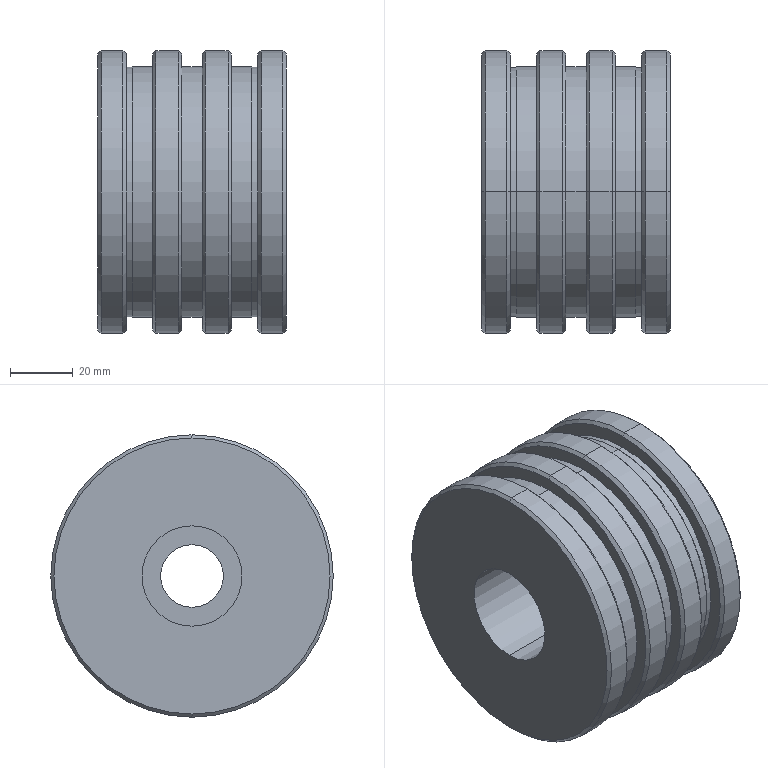Part | SolidWorks | features Chamfer 1, Revolution 1 | 1 solid | 52 faces | box 60 x 90 x 90 mm | volume 271909 mm3 | cylinder 24 | cone 16 | plane 12 | commonest cylinder face diameters 90 x8 80 x6 79.6 x4 20 x2 32 x2 64 x2
STEP:
#1=CARTESIAN_POINT('',(0.,0.,44.));
#2=VERTEX_POINT('',#1);
#3=CARTESIAN_POINT('',(0.,0.,-44.));
#4=VERTEX_POINT('',#3);
#5=CARTESIAN_POINT('',(0.,0.,0.));
#6=DIRECTION('',(-1.,0.,0.));
#7=DIRECTION('',(0.,0.,-1.));
#8=AXIS2_PLACEMENT_3D('',#5,#6,#7);
#9=CIRCLE('',#8,44.);
#10=EDGE_CURVE('',#2,#4,#9,.T.);
#11=ORIENTED_EDGE('',*,*,#10,.F.);
#12=CARTESIAN_POINT('',(1.,0.,45.));
#13=VERTEX_POINT('',#12);
#14=CARTESIAN_POINT('',(0.,0.,44.));
#15=DIRECTION('',(0.7071,0.,0.7071));
#16=VECTOR('',#15,1000.);
#17=LINE('',#14,#16);
#18=EDGE_CURVE('',#2,#13,#17,.T.);
#19=ORIENTED_EDGE('',*,*,#18,.T.);
#20=CARTESIAN_POINT('',(1.,0.,-45.));
#21=VERTEX_POINT('',#20);
#22=CARTESIAN_POINT('',(1.,0.,0.));
#23=DIRECTION('',(1.,0.,0.));
#24=DIRECTION('',(0.,0.,-1.));
#25=AXIS2_PLACEMENT_3D('',#22,#23,#24);
#26=CIRCLE('',#25,45.);
#27=EDGE_CURVE('',#21,#13,#26,.T.);
#28=ORIENTED_EDGE('',*,*,#27,.F.);
#29=CARTESIAN_POINT('',(0.,0.,-44.));
#30=DIRECTION('',(0.7071,0.,-0.7071));
#31=VECTOR('',#30,1000.);
#32=LINE('',#29,#31);
#33=EDGE_CURVE('',#4,#21,#32,.T.);
#34=ORIENTED_EDGE('',*,*,#33,.F.);
#35=EDGE_LOOP('',(#11,#19,#28,#34));
#36=FACE_OUTER_BOUND('',#35,.T.);
#37=CARTESIAN_POINT('',(0.,0.,0.));
#38=DIRECTION('',(1.,0.,0.));
#39=DIRECTION('',(0.,0.,-1.));
#40=AXIS2_PLACEMENT_3D('',#37,#38,#39);
#41=CONICAL_SURFACE('',#40,44.,0.7854);
#42=ADVANCED_FACE('',(#36),#41,.T.);
#43=CARTESIAN_POINT('',(9.,0.,-44.));
#44=VERTEX_POINT('',#43);
#45=CARTESIAN_POINT('',(9.,0.,44.));
#46=VERTEX_POINT('',#45);
#47=CARTESIAN_POINT('',(9.,0.,0.));
#48=DIRECTION('',(1.,0.,0.));
#49=DIRECTION('',(0.,0.,1.));
#50=AXIS2_PLACEMENT_3D('',#47,#48,#49);
#51=CIRCLE('',#50,44.);
#52=EDGE_CURVE('',#44,#46,#51,.T.);
#53=ORIENTED_EDGE('',*,*,#52,.F.);
#54=CARTESIAN_POINT('',(8.,0.,-45.));
#55=VERTEX_POINT('',#54);
#56=CARTESIAN_POINT('',(8.,0.,-45.));
#57=DIRECTION('',(-0.7071,0.,-0.7071));
#58=VECTOR('',#57,1000.);
#59=LINE('',#56,#58);
#60=EDGE_CURVE('',#44,#55,#59,.T.);
#61=ORIENTED_EDGE('',*,*,#60,.T.);
#62=CARTESIAN_POINT('',(8.,0.,45.));
#63=VERTEX_POINT('',#62);
#64=CARTESIAN_POINT('',(8.,0.,0.));
#65=DIRECTION('',(-1.,0.,0.));
#66=DIRECTION('',(0.,0.,1.));
#67=AXIS2_PLACEMENT_3D('',#64,#65,#66);
#68=CIRCLE('',#67,45.);
#69=EDGE_CURVE('',#63,#55,#68,.T.);
#70=ORIENTED_EDGE('',*,*,#69,.F.);
#71=CARTESIAN_POINT('',(8.,0.,45.));
#72=DIRECTION('',(-0.7071,0.,0.7071));
#73=VECTOR('',#72,1000.);
#74=LINE('',#71,#73);
#75=EDGE_CURVE('',#46,#63,#74,.T.);
#76=ORIENTED_EDGE('',*,*,#75,.F.);
#77=EDGE_LOOP('',(#53,#61,#70,#76));
#78=FACE_OUTER_BOUND('',#77,.T.);
#79=CARTESIAN_POINT('',(8.,0.,0.));
#80=DIRECTION('',(-1.,0.,0.));
#81=DIRECTION('',(0.,0.,1.));
#82=AXIS2_PLACEMENT_3D('',#79,#80,#81);
#83=CONICAL_SURFACE('',#82,45.,0.7854);
#84=ADVANCED_FACE('',(#78),#83,.T.);
#85=CARTESIAN_POINT('',(17.5,0.,44.));
#86=VERTEX_POINT('',#85);
#87=CARTESIAN_POINT('',(17.5,0.,-44.));
#88=VERTEX_POINT('',#87);
#89=CARTESIAN_POINT('',(17.5,0.,0.));
#90=DIRECTION('',(-1.,0.,0.));
#91=DIRECTION('',(0.,0.,-1.));
#92=AXIS2_PLACEMENT_3D('',#89,#90,#91);
#93=CIRCLE('',#92,44.);
#94=EDGE_CURVE('',#86,#88,#93,.T.);
#95=ORIENTED_EDGE('',*,*,#94,.F.);
#96=CARTESIAN_POINT('',(18.5,0.,45.));
#97=VERTEX_POINT('',#96);
#98=CARTESIAN_POINT('',(17.5,0.,44.));
#99=DIRECTION('',(0.7071,0.,0.7071));
#100=VECTOR('',#99,1000.);
#101=LINE('',#98,#100);
#102=EDGE_CURVE('',#86,#97,#101,.T.);
#103=ORIENTED_EDGE('',*,*,#102,.T.);
#104=CARTESIAN_POINT('',(18.5,0.,-45.));
#105=VERTEX_POINT('',#104);
#106=CARTESIAN_POINT('',(18.5,0.,0.));
#107=DIRECTION('',(1.,0.,0.));
#108=DIRECTION('',(0.,0.,-1.));
#109=AXIS2_PLACEMENT_3D('',#106,#107,#108);
#110=CIRCLE('',#109,45.);
#111=EDGE_CURVE('',#105,#97,#110,.T.);
#112=ORIENTED_EDGE('',*,*,#111,.F.);
#113=CARTESIAN_POINT('',(17.5,0.,-44.));
#114=DIRECTION('',(0.7071,0.,-0.7071));
#115=VECTOR('',#114,1000.);
#116=LINE('',#113,#115);
#117=EDGE_CURVE('',#88,#105,#116,.T.);
#118=ORIENTED_EDGE('',*,*,#117,.F.);
#119=EDGE_LOOP('',(#95,#103,#112,#118));
#120=FACE_OUTER_BOUND('',#119,.T.);
#121=CARTESIAN_POINT('',(17.5,0.,0.));
#122=DIRECTION('',(1.,0.,0.));
#123=DIRECTION('',(0.,0.,-1.));
#124=AXIS2_PLACEMENT_3D('',#121,#122,#123);
#125=CONICAL_SURFACE('',#124,44.,0.7854);
#126=ADVANCED_FACE('',(#120),#125,.T.);
#127=CARTESIAN_POINT('',(26.75,0.,-44.));
#128=VERTEX_POINT('',#127);
#129=CARTESIAN_POINT('',(26.75,0.,44.));
#130=VERTEX_POINT('',#129);
#131=CARTESIAN_POINT('',(26.75,0.,0.));
#132=DIRECTION('',(1.,0.,0.));
#133=DIRECTION('',(0.,0.,1.));
#134=AXIS2_PLACEMENT_3D('',#131,#132,#133);
#135=CIRCLE('',#134,44.);
#136=EDGE_CURVE('',#128,#130,#135,.T.);
#137=ORIENTED_EDGE('',*,*,#136,.F.);
#138=CARTESIAN_POINT('',(25.75,0.,-45.));
#139=VERTEX_POINT('',#138);
#140=CARTESIAN_POINT('',(25.75,0.,-45.));
#141=DIRECTION('',(-0.7071,0.,-0.7071));
#142=VECTOR('',#141,1000.);
#143=LINE('',#140,#142);
#144=EDGE_CURVE('',#128,#139,#143,.T.);
#145=ORIENTED_EDGE('',*,*,#144,.T.);
#146=CARTESIAN_POINT('',(25.75,0.,45.));
#147=VERTEX_POINT('',#146);
#148=CARTESIAN_POINT('',(25.75,0.,0.));
#149=DIRECTION('',(-1.,0.,0.));
#150=DIRECTION('',(0.,0.,1.));
#151=AXIS2_PLACEMENT_3D('',#148,#149,#150);
#152=CIRCLE('',#151,45.);
#153=EDGE_CURVE('',#147,#139,#152,.T.);
#154=ORIENTED_EDGE('',*,*,#153,.F.);
#155=CARTESIAN_POINT('',(25.75,0.,45.));
#156=DIRECTION('',(-0.7071,0.,0.7071));
#157=VECTOR('',#156,1000.);
#158=LINE('',#155,#157);
#159=EDGE_CURVE('',#130,#147,#158,.T.);
#160=ORIENTED_EDGE('',*,*,#159,.F.);
#161=EDGE_LOOP('',(#137,#145,#154,#160));
#162=FACE_OUTER_BOUND('',#161,.T.);
#163=CARTESIAN_POINT('',(25.75,0.,0.));
#164=DIRECTION('',(-1.,0.,0.));
#165=DIRECTION('',(0.,0.,1.));
#166=AXIS2_PLACEMENT_3D('',#163,#164,#165);
#167=CONICAL_SURFACE('',#166,45.,0.7854);
#168=ADVANCED_FACE('',(#162),#167,.T.);
#169=CARTESIAN_POINT('',(33.25,0.,44.));
#170=VERTEX_POINT('',#169);
#171=CARTESIAN_POINT('',(33.25,0.,-44.));
#172=VERTEX_POINT('',#171);
#173=CARTESIAN_POINT('',(33.25,0.,0.));
#174=DIRECTION('',(-1.,0.,0.));
#175=DIRECTION('',(0.,0.,-1.));
#176=AXIS2_PLACEMENT_3D('',#173,#174,#175);
#177=CIRCLE('',#176,44.);
#178=EDGE_CURVE('',#170,#172,#177,.T.);
#179=ORIENTED_EDGE('',*,*,#178,.F.);
#180=CARTESIAN_POINT('',(34.25,0.,45.));
#181=VERTEX_POINT('',#180);
#182=CARTESIAN_POINT('',(33.25,0.,44.));
#183=DIRECTION('',(0.7071,0.,0.7071));
#184=VECTOR('',#183,1000.);
#185=LINE('',#182,#184);
#186=EDGE_CURVE('',#170,#181,#185,.T.);
#187=ORIENTED_EDGE('',*,*,#186,.T.);
#188=CARTESIAN_POINT('',(34.25,0.,-45.));
#189=VERTEX_POINT('',#188);
#190=CARTESIAN_POINT('',(34.25,0.,0.));
#191=DIRECTION('',(1.,0.,0.));
#192=DIRECTION('',(0.,0.,-1.));
#193=AXIS2_PLACEMENT_3D('',#190,#191,#192);
#194=CIRCLE('',#193,45.);
#195=EDGE_CURVE('',#189,#181,#194,.T.);
#196=ORIENTED_EDGE('',*,*,#195,.F.);
#197=CARTESIAN_POINT('',(33.25,0.,-44.));
#198=DIRECTION('',(0.7071,0.,-0.7071));
#199=VECTOR('',#198,1000.);
#200=LINE('',#197,#199);
#201=EDGE_CURVE('',#172,#189,#200,.T.);
#202=ORIENTED_EDGE('',*,*,#201,.F.);
#203=EDGE_LOOP('',(#179,#187,#196,#202));
#204=FACE_OUTER_BOUND('',#203,.T.);
#205=CARTESIAN_POINT('',(33.25,0.,0.));
#206=DIRECTION('',(1.,0.,0.));
#207=DIRECTION('',(0.,0.,-1.));
#208=AXIS2_PLACEMENT_3D('',#205,#206,#207);
#209=CONICAL_SURFACE('',#208,44.,0.7854);
#210=ADVANCED_FACE('',(#204),#209,.T.);
#211=CARTESIAN_POINT('',(42.5,0.,-44.));
#212=VERTEX_POINT('',#211);
#213=CARTESIAN_POINT('',(42.5,0.,44.));
#214=VERTEX_POINT('',#213);
#215=CARTESIAN_POINT('',(42.5,0.,0.));
#216=DIRECTION('',(1.,0.,0.));
#217=DIRECTION('',(0.,0.,1.));
#218=AXIS2_PLACEMENT_3D('',#215,#216,#217);
#219=CIRCLE('',#218,44.);
#220=EDGE_CURVE('',#212,#214,#219,.T.);
#221=ORIENTED_EDGE('',*,*,#220,.F.);
#222=CARTESIAN_POINT('',(41.5,0.,-45.));
#223=VERTEX_POINT('',#222);
#224=CARTESIAN_POINT('',(41.5,0.,-45.));
#225=DIRECTION('',(-0.7071,0.,-0.7071));
#226=VECTOR('',#225,1000.);
#227=LINE('',#224,#226);
#228=EDGE_CURVE('',#212,#223,#227,.T.);
#229=ORIENTED_EDGE('',*,*,#228,.T.);
#230=CARTESIAN_POINT('',(41.5,0.,45.));
#231=VERTEX_POINT('',#230);
#232=CARTESIAN_POINT('',(41.5,0.,0.));
#233=DIRECTION('',(-1.,0.,0.));
#234=DIRECTION('',(0.,0.,1.));
#235=AXIS2_PLACEMENT_3D('',#232,#233,#234);
#236=CIRCLE('',#235,45.);
#237=EDGE_CURVE('',#231,#223,#236,.T.);
#238=ORIENTED_EDGE('',*,*,#237,.F.);
#239=CARTESIAN_POINT('',(41.5,0.,45.));
#240=DIRECTION('',(-0.7071,0.,0.7071));
#241=VECTOR('',#240,1000.);
#242=LINE('',#239,#241);
#243=EDGE_CURVE('',#214,#231,#242,.T.);
#244=ORIENTED_EDGE('',*,*,#243,.F.);
#245=EDGE_LOOP('',(#221,#229,#238,#244));
#246=FACE_OUTER_BOUND('',#245,.T.);
#247=CARTESIAN_POINT('',(41.5,0.,0.));
#248=DIRECTION('',(-1.,0.,0.));
#249=DIRECTION('',(0.,0.,1.));
#250=AXIS2_PLACEMENT_3D('',#247,#248,#249);
#251=CONICAL_SURFACE('',#250,45.,0.7854);
#252=ADVANCED_FACE('',(#246),#251,.T.);
#253=CARTESIAN_POINT('',(51.,0.,44.));
#254=VERTEX_POINT('',#253);
#255=CARTESIAN_POINT('',(51.,0.,-44.));
#256=VERTEX_POINT('',#255);
#257=CARTESIAN_POINT('',(51.,0.,0.));
#258=DIRECTION('',(-1.,0.,0.));
#259=DIRECTION('',(0.,0.,-1.));
#260=AXIS2_PLACEMENT_3D('',#257,#258,#259);
#261=CIRCLE('',#260,44.);
#262=EDGE_CURVE('',#254,#256,#261,.T.);
#263=ORIENTED_EDGE('',*,*,#262,.F.);
#264=CARTESIAN_POINT('',(52.,0.,45.));
#265=VERTEX_POINT('',#264);
#266=CARTESIAN_POINT('',(51.,0.,44.));
#267=DIRECTION('',(0.7071,0.,0.7071));
#268=VECTOR('',#267,1000.);
#269=LINE('',#266,#268);
#270=EDGE_CURVE('',#254,#265,#269,.T.);
#271=ORIENTED_EDGE('',*,*,#270,.T.);
#272=CARTESIAN_POINT('',(52.,0.,-45.));
#273=VERTEX_POINT('',#272);
#274=CARTESIAN_POINT('',(52.,0.,0.));
#275=DIRECTION('',(1.,0.,0.));
#276=DIRECTION('',(0.,0.,-1.));
#277=AXIS2_PLACEMENT_3D('',#274,#275,#276);
#278=CIRCLE('',#277,45.);
#279=EDGE_CURVE('',#273,#265,#278,.T.);
#280=ORIENTED_EDGE('',*,*,#279,.F.);
#281=CARTESIAN_POINT('',(51.,0.,-44.));
#282=DIRECTION('',(0.7071,0.,-0.7071));
#283=VECTOR('',#282,1000.);
#284=LINE('',#281,#283);
#285=EDGE_CURVE('',#256,#273,#284,.T.);
#286=ORIENTED_EDGE('',*,*,#285,.F.);
#287=EDGE_LOOP('',(#263,#271,#280,#286));
#288=FACE_OUTER_BOUND('',#287,.T.);
#289=CARTESIAN_POINT('',(51.,0.,0.));
#290=DIRECTION('',(1.,0.,0.));
#291=DIRECTION('',(0.,0.,-1.));
#292=AXIS2_PLACEMENT_3D('',#289,#290,#291);
#293=CONICAL_SURFACE('',#292,44.,0.7854);
#294=ADVANCED_FACE('',(#288),#293,.T.);
#295=CARTESIAN_POINT('',(60.,0.,-44.));
#296=VERTEX_POINT('',#295);
#297=CARTESIAN_POINT('',(60.,0.,44.));
#298=VERTEX_POINT('',#297);
#299=CARTESIAN_POINT('',(60.,0.,0.));
#300=DIRECTION('',(1.,0.,0.));
#301=DIRECTION('',(0.,0.,1.));
#302=AXIS2_PLACEMENT_3D('',#299,#300,#301);
#303=CIRCLE('',#302,44.);
#304=EDGE_CURVE('',#296,#298,#303,.T.);
#305=ORIENTED_EDGE('',*,*,#304,.F.);
#306=CARTESIAN_POINT('',(59.,0.,-45.));
#307=VERTEX_POINT('',#306);
#308=CARTESIAN_POINT('',(59.,0.,-45.));
#309=DIRECTION('',(-0.7071,0.,-0.7071));
#310=VECTOR('',#309,1000.);
#311=LINE('',#308,#310);
#312=EDGE_CURVE('',#296,#307,#311,.T.);
#313=ORIENTED_EDGE('',*,*,#312,.T.);
#314=CARTESIAN_POINT('',(59.,0.,45.));
#315=VERTEX_POINT('',#314);
#316=CARTESIAN_POINT('',(59.,0.,0.));
#317=DIRECTION('',(-1.,0.,0.));
#318=DIRECTION('',(0.,0.,1.));
#319=AXIS2_PLACEMENT_3D('',#316,#317,#318);
#320=CIRCLE('',#319,45.);
#321=EDGE_CURVE('',#315,#307,#320,.T.);
#322=ORIENTED_EDGE('',*,*,#321,.F.);
#323=CARTESIAN_POINT('',(59.,0.,45.));
#324=DIRECTION('',(-0.7071,0.,0.7071));
#325=VECTOR('',#324,1000.);
#326=LINE('',#323,#325);
#327=EDGE_CURVE('',#298,#315,#326,.T.);
#328=ORIENTED_EDGE('',*,*,#327,.F.);
#329=EDGE_LOOP('',(#305,#313,#322,#328));
#330=FACE_OUTER_BOUND('',#329,.T.);
#331=CARTESIAN_POINT('',(59.,0.,0.));
#332=DIRECTION('',(-1.,0.,0.));
#333=DIRECTION('',(0.,0.,1.));
#334=AXIS2_PLACEMENT_3D('',#331,#332,#333);
#335=CONICAL_SURFACE('',#334,45.,0.7854);
#336=ADVANCED_FACE('',(#330),#335,.T.);
#337=CARTESIAN_POINT('',(45.,0.,-10.));
#338=VERTEX_POINT('',#337);
#339=CARTESIAN_POINT('',(45.,0.,10.));
#340=VERTEX_POINT('',#339);
#341=CARTESIAN_POINT('',(45.,0.,0.));
#342=DIRECTION('',(-1.,0.,0.));
#343=DIRECTION('',(0.,0.,1.));
#344=AXIS2_PLACEMENT_3D('',#341,#342,#343);
#345=CIRCLE('',#344,10.);
#346=EDGE_CURVE('',#338,#340,#345,.T.);
#347=ORIENTED_EDGE('',*,*,#346,.F.);
#348=CARTESIAN_POINT('',(30.,0.,-10.));
#349=VERTEX_POINT('',#348);
#350=CARTESIAN_POINT('',(0.,0.,-10.));
#351=DIRECTION('',(-1.,0.,0.));
#352=VECTOR('',#351,1000.);
#353=LINE('',#350,#352);
#354=EDGE_CURVE('',#338,#349,#353,.T.);
#355=ORIENTED_EDGE('',*,*,#354,.T.);
#356=CARTESIAN_POINT('',(30.,0.,10.));
#357=VERTEX_POINT('',#356);
#358=CARTESIAN_POINT('',(30.,0.,0.));
#359=DIRECTION('',(-1.,0.,0.));
#360=DIRECTION('',(0.,0.,1.));
#361=AXIS2_PLACEMENT_3D('',#358,#359,#360);
#362=CIRCLE('',#361,10.);
#363=EDGE_CURVE('',#349,#357,#362,.T.);
#364=ORIENTED_EDGE('',*,*,#363,.T.);
#365=CARTESIAN_POINT('',(0.,0.,10.));
#366=DIRECTION('',(-1.,0.,0.));
#367=VECTOR('',#366,1000.);
#368=LINE('',#365,#367);
#369=EDGE_CURVE('',#340,#357,#368,.T.);
#370=ORIENTED_EDGE('',*,*,#369,.F.);
#371=EDGE_LOOP('',(#347,#355,#364,#370));
#372=FACE_OUTER_BOUND('',#371,.T.);
#373=CARTESIAN_POINT('',(0.,0.,0.));
#374=DIRECTION('',(-1.,0.,0.));
#375=DIRECTION('',(0.,0.,1.));
#376=AXIS2_PLACEMENT_3D('',#373,#374,#375);
#377=CYLINDRICAL_SURFACE('',#376,10.);
#378=ADVANCED_FACE('',(#372),#377,.F.);
#379=CARTESIAN_POINT('',(60.,0.,-32.));
#380=VERTEX_POINT('',#379);
#381=CARTESIAN_POINT('',(60.,0.,32.));
#382=VERTEX_POINT('',#381);
#383=CARTESIAN_POINT('',(60.,0.,0.));
#384=DIRECTION('',(-1.,0.,0.));
#385=DIRECTION('',(0.,0.,1.));
#386=AXIS2_PLACEMENT_3D('',#383,#384,#385);
#387=CIRCLE('',#386,32.);
#388=EDGE_CURVE('',#380,#382,#387,.T.);
#389=ORIENTED_EDGE('',*,*,#388,.F.);
#390=CARTESIAN_POINT('',(45.,0.,-32.));
#391=VERTEX_POINT('',#390);
#392=CARTESIAN_POINT('',(0.,0.,-32.));
#393=DIRECTION('',(-1.,0.,0.));
#394=VECTOR('',#393,1000.);
#395=LINE('',#392,#394);
#396=EDGE_CURVE('',#380,#391,#395,.T.);
#397=ORIENTED_EDGE('',*,*,#396,.T.);
#398=CARTESIAN_POINT('',(45.,0.,32.));
#399=VERTEX_POINT('',#398);
#400=CARTESIAN_POINT('',(45.,0.,0.));
#401=DIRECTION('',(-1.,0.,0.));
#402=DIRECTION('',(0.,0.,1.));
#403=AXIS2_PLACEMENT_3D('',#400,#401,#402);
#404=CIRCLE('',#403,32.);
#405=EDGE_CURVE('',#391,#399,#404,.T.);
#406=ORIENTED_EDGE('',*,*,#405,.T.);
#407=CARTESIAN_POINT('',(0.,0.,32.));
#408=DIRECTION('',(-1.,0.,0.));
#409=VECTOR('',#408,1000.);
#410=LINE('',#407,#409);
#411=EDGE_CURVE('',#382,#399,#410,.T.);
#412=ORIENTED_EDGE('',*,*,#411,.F.);
#413=EDGE_LOOP('',(#389,#397,#406,#412));
#414=FACE_OUTER_BOUND('',#413,.T.);
#415=CARTESIAN_POINT('',(0.,0.,0.));
#416=DIRECTION('',(-1.,0.,0.));
#417=DIRECTION('',(0.,0.,1.));
#418=AXIS2_PLACEMENT_3D('',#415,#416,#417);
#419=CYLINDRICAL_SURFACE('',#418,32.);
#420=ADVANCED_FACE('',(#414),#419,.F.);
#421=ORIENTED_EDGE('',*,*,#321,.T.);
#422=CARTESIAN_POINT('',(0.,0.,-45.));
#423=DIRECTION('',(-1.,0.,0.));
#424=VECTOR('',#423,1000.);
#425=LINE('',#422,#424);
#426=EDGE_CURVE('',#307,#273,#425,.T.);
#427=ORIENTED_EDGE('',*,*,#426,.T.);
#428=ORIENTED_EDGE('',*,*,#279,.T.);
#429=CARTESIAN_POINT('',(0.,0.,45.));
#430=DIRECTION('',(-1.,0.,0.));
#431=VECTOR('',#430,1000.);
#432=LINE('',#429,#431);
#433=EDGE_CURVE('',#315,#265,#432,.T.);
#434=ORIENTED_EDGE('',*,*,#433,.F.);
#435=EDGE_LOOP('',(#421,#427,#428,#434));
#436=FACE_OUTER_BOUND('',#435,.T.);
#437=CARTESIAN_POINT('',(0.,0.,0.));
#438=DIRECTION('',(-1.,0.,0.));
#439=DIRECTION('',(0.,0.,1.));
#440=AXIS2_PLACEMENT_3D('',#437,#438,#439);
#441=CYLINDRICAL_SURFACE('',#440,45.);
#442=ADVANCED_FACE('',(#436),#441,.T.);
#443=CARTESIAN_POINT('',(51.,0.,39.8));
#444=VERTEX_POINT('',#443);
#445=CARTESIAN_POINT('',(51.,0.,-39.8));
#446=VERTEX_POINT('',#445);
#447=CARTESIAN_POINT('',(51.,0.,0.));
#448=DIRECTION('',(-1.,0.,0.));
#449=DIRECTION('',(0.,0.,1.));
#450=AXIS2_PLACEMENT_3D('',#447,#448,#449);
#451=CIRCLE('',#450,39.8);
#452=EDGE_CURVE('',#444,#446,#451,.T.);
#453=ORIENTED_EDGE('',*,*,#452,.T.);
#454=CARTESIAN_POINT('',(49.,0.,-39.8));
#455=VERTEX_POINT('',#454);
#456=CARTESIAN_POINT('',(0.,0.,-39.8));
#457=DIRECTION('',(-1.,0.,0.));
#458=VECTOR('',#457,1000.);
#459=LINE('',#456,#458);
#460=EDGE_CURVE('',#446,#455,#459,.T.);
#461=ORIENTED_EDGE('',*,*,#460,.T.);
#462=CARTESIAN_POINT('',(49.,0.,39.8));
#463=VERTEX_POINT('',#462);
#464=CARTESIAN_POINT('',(49.,0.,0.));
#465=DIRECTION('',(-1.,0.,0.));
#466=DIRECTION('',(0.,0.,1.));
#467=AXIS2_PLACEMENT_3D('',#464,#465,#466);
#468=CIRCLE('',#467,39.8);
#469=EDGE_CURVE('',#463,#455,#468,.T.);
#470=ORIENTED_EDGE('',*,*,#469,.F.);
#471=CARTESIAN_POINT('',(0.,0.,39.8));
#472=DIRECTION('',(-1.,0.,0.));
#473=VECTOR('',#472,1000.);
#474=LINE('',#471,#473);
#475=EDGE_CURVE('',#444,#463,#474,.T.);
#476=ORIENTED_EDGE('',*,*,#475,.F.);
#477=EDGE_LOOP('',(#453,#461,#470,#476));
#478=FACE_OUTER_BOUND('',#477,.T.);
#479=CARTESIAN_POINT('',(0.,0.,0.));
#480=DIRECTION('',(-1.,0.,0.));
#481=DIRECTION('',(0.,0.,1.));
#482=AXIS2_PLACEMENT_3D('',#479,#480,#481);
#483=CYLINDRICAL_SURFACE('',#482,39.8);
#484=ADVANCED_FACE('',(#478),#483,.T.);
#485=CARTESIAN_POINT('',(49.,0.,40.));
#486=VERTEX_POINT('',#485);
#487=CARTESIAN_POINT('',(49.,0.,-40.));
#488=VERTEX_POINT('',#487);
#489=CARTESIAN_POINT('',(49.,0.,0.));
#490=DIRECTION('',(-1.,0.,0.));
#491=DIRECTION('',(0.,0.,1.));
#492=AXIS2_PLACEMENT_3D('',#489,#490,#491);
#493=CIRCLE('',#492,40.);
#494=EDGE_CURVE('',#486,#488,#493,.T.);
#495=ORIENTED_EDGE('',*,*,#494,.T.);
#496=CARTESIAN_POINT('',(42.5,0.,-40.));
#497=VERTEX_POINT('',#496);
#498=CARTESIAN_POINT('',(0.,0.,-40.));
#499=DIRECTION('',(-1.,0.,0.));
#500=VECTOR('',#499,1000.);
#501=LINE('',#498,#500);
#502=EDGE_CURVE('',#488,#497,#501,.T.);
#503=ORIENTED_EDGE('',*,*,#502,.T.);
#504=CARTESIAN_POINT('',(42.5,0.,40.));
#505=VERTEX_POINT('',#504);
#506=CARTESIAN_POINT('',(42.5,0.,0.));
#507=DIRECTION('',(-1.,0.,0.));
#508=DIRECTION('',(0.,0.,1.));
#509=AXIS2_PLACEMENT_3D('',#506,#507,#508);
#510=CIRCLE('',#509,40.);
#511=EDGE_CURVE('',#505,#497,#510,.T.);
#512=ORIENTED_EDGE('',*,*,#511,.F.);
#513=CARTESIAN_POINT('',(0.,0.,40.));
#514=DIRECTION('',(-1.,0.,0.));
#515=VECTOR('',#514,1000.);
#516=LINE('',#513,#515);
#517=EDGE_CURVE('',#486,#505,#516,.T.);
#518=ORIENTED_EDGE('',*,*,#517,.F.);
#519=EDGE_LOOP('',(#495,#503,#512,#518));
#520=FACE_OUTER_BOUND('',#519,.T.);
#521=CARTESIAN_POINT('',(0.,0.,0.));
#522=DIRECTION('',(-1.,0.,0.));
#523=DIRECTION('',(0.,0.,1.));
#524=AXIS2_PLACEMENT_3D('',#521,#522,#523);
#525=CYLINDRICAL_SURFACE('',#524,40.);
#526=ADVANCED_FACE('',(#520),#525,.T.);
#527=ORIENTED_EDGE('',*,*,#237,.T.);
#528=CARTESIAN_POINT('',(0.,0.,-45.));
#529=DIRECTION('',(-1.,0.,0.));
#530=VECTOR('',#529,1000.);
#531=LINE('',#528,#530);
#532=EDGE_CURVE('',#223,#189,#531,.T.);
#533=ORIENTED_EDGE('',*,*,#532,.T.);
#534=ORIENTED_EDGE('',*,*,#195,.T.);
#535=CARTESIAN_POINT('',(0.,0.,45.));
#536=DIRECTION('',(-1.,0.,0.));
#537=VECTOR('',#536,1000.);
#538=LINE('',#535,#537);
#539=EDGE_CURVE('',#231,#181,#538,.T.);
#540=ORIENTED_EDGE('',*,*,#539,.F.);
#541=EDGE_LOOP('',(#527,#533,#534,#540));
#542=FACE_OUTER_BOUND('',#541,.T.);
#543=CARTESIAN_POINT('',(0.,0.,0.));
#544=DIRECTION('',(-1.,0.,0.));
#545=DIRECTION('',(0.,0.,1.));
#546=AXIS2_PLACEMENT_3D('',#543,#544,#545);
#547=CYLINDRICAL_SURFACE('',#546,45.);
#548=ADVANCED_FACE('',(#542),#547,.T.);
#549=CARTESIAN_POINT('',(33.25,0.,40.));
#550=VERTEX_POINT('',#549);
#551=CARTESIAN_POINT('',(33.25,0.,-40.));
#552=VERTEX_POINT('',#551);
#553=CARTESIAN_POINT('',(33.25,0.,0.));
#554=DIRECTION('',(-1.,0.,0.));
#555=DIRECTION('',(0.,0.,1.));
#556=AXIS2_PLACEMENT_3D('',#553,#554,#555);
#557=CIRCLE('',#556,40.);
#558=EDGE_CURVE('',#550,#552,#557,.T.);
#559=ORIENTED_EDGE('',*,*,#558,.T.);
#560=CARTESIAN_POINT('',(26.75,0.,-40.));
#561=VERTEX_POINT('',#560);
#562=CARTESIAN_POINT('',(0.,0.,-40.));
#563=DIRECTION('',(-1.,0.,0.));
#564=VECTOR('',#563,1000.);
#565=LINE('',#562,#564);
#566=EDGE_CURVE('',#552,#561,#565,.T.);
#567=ORIENTED_EDGE('',*,*,#566,.T.);
#568=CARTESIAN_POINT('',(26.75,0.,40.));
#569=VERTEX_POINT('',#568);
#570=CARTESIAN_POINT('',(26.75,0.,0.));
#571=DIRECTION('',(-1.,0.,0.));
#572=DIRECTION('',(0.,0.,1.));
#573=AXIS2_PLACEMENT_3D('',#570,#571,#572);
#574=CIRCLE('',#573,40.);
#575=EDGE_CURVE('',#569,#561,#574,.T.);
#576=ORIENTED_EDGE('',*,*,#575,.F.);
#577=CARTESIAN_POINT('',(0.,0.,40.));
#578=DIRECTION('',(-1.,0.,0.));
#579=VECTOR('',#578,1000.);
#580=LINE('',#577,#579);
#581=EDGE_CURVE('',#550,#569,#580,.T.);
#582=ORIENTED_EDGE('',*,*,#581,.F.);
#583=EDGE_LOOP('',(#559,#567,#576,#582));
#584=FACE_OUTER_BOUND('',#583,.T.);
#585=CARTESIAN_POINT('',(0.,0.,0.));
#586=DIRECTION('',(-1.,0.,0.));
#587=DIRECTION('',(0.,0.,1.));
#588=AXIS2_PLACEMENT_3D('',#585,#586,#587);
#589=CYLINDRICAL_SURFACE('',#588,40.);
#590=ADVANCED_FACE('',(#584),#589,.T.);
#591=ORIENTED_EDGE('',*,*,#153,.T.);
#592=CARTESIAN_POINT('',(0.,0.,-45.));
#593=DIRECTION('',(-1.,0.,0.));
#594=VECTOR('',#593,1000.);
#595=LINE('',#592,#594);
#596=EDGE_CURVE('',#139,#105,#595,.T.);
#597=ORIENTED_EDGE('',*,*,#596,.T.);
#598=ORIENTED_EDGE('',*,*,#111,.T.);
#599=CARTESIAN_POINT('',(0.,0.,45.));
#600=DIRECTION('',(-1.,0.,0.));
#601=VECTOR('',#600,1000.);
#602=LINE('',#599,#601);
#603=EDGE_CURVE('',#147,#97,#602,.T.);
#604=ORIENTED_EDGE('',*,*,#603,.F.);
#605=EDGE_LOOP('',(#591,#597,#598,#604));
#606=FACE_OUTER_BOUND('',#605,.T.);
#607=CARTESIAN_POINT('',(0.,0.,0.));
#608=DIRECTION('',(-1.,0.,0.));
#609=DIRECTION('',(0.,0.,1.));
#610=AXIS2_PLACEMENT_3D('',#607,#608,#609);
#611=CYLINDRICAL_SURFACE('',#610,45.);
#612=ADVANCED_FACE('',(#606),#611,.T.);
#613=CARTESIAN_POINT('',(17.5,0.,40.));
#614=VERTEX_POINT('',#613);
#615=CARTESIAN_POINT('',(17.5,0.,-40.));
#616=VERTEX_POINT('',#615);
#617=CARTESIAN_POINT('',(17.5,0.,0.));
#618=DIRECTION('',(-1.,0.,0.));
#619=DIRECTION('',(0.,0.,1.));
#620=AXIS2_PLACEMENT_3D('',#617,#618,#619);
#621=CIRCLE('',#620,40.);
#622=EDGE_CURVE('',#614,#616,#621,.T.);
#623=ORIENTED_EDGE('',*,*,#622,.T.);
#624=CARTESIAN_POINT('',(11.,0.,-40.));
#625=VERTEX_POINT('',#624);
#626=CARTESIAN_POINT('',(0.,0.,-40.));
#627=DIRECTION('',(-1.,0.,0.));
#628=VECTOR('',#627,1000.);
#629=LINE('',#626,#628);
#630=EDGE_CURVE('',#616,#625,#629,.T.);
#631=ORIENTED_EDGE('',*,*,#630,.T.);
#632=CARTESIAN_POINT('',(11.,0.,40.));
#633=VERTEX_POINT('',#632);
#634=CARTESIAN_POINT('',(11.,0.,0.));
#635=DIRECTION('',(-1.,0.,0.));
#636=DIRECTION('',(0.,0.,1.));
#637=AXIS2_PLACEMENT_3D('',#634,#635,#636);
#638=CIRCLE('',#637,40.);
#639=EDGE_CURVE('',#633,#625,#638,.T.);
#640=ORIENTED_EDGE('',*,*,#639,.F.);
#641=CARTESIAN_POINT('',(0.,0.,40.));
#642=DIRECTION('',(-1.,0.,0.));
#643=VECTOR('',#642,1000.);
#644=LINE('',#641,#643);
#645=EDGE_CURVE('',#614,#633,#644,.T.);
#646=ORIENTED_EDGE('',*,*,#645,.F.);
#647=EDGE_LOOP('',(#623,#631,#640,#646));
#648=FACE_OUTER_BOUND('',#647,.T.);
#649=CARTESIAN_POINT('',(0.,0.,0.));
#650=DIRECTION('',(-1.,0.,0.));
#651=DIRECTION('',(0.,0.,1.));
#652=AXIS2_PLACEMENT_3D('',#649,#650,#651);
#653=CYLINDRICAL_SURFACE('',#652,40.);
#654=ADVANCED_FACE('',(#648),#653,.T.);
#655=CARTESIAN_POINT('',(11.,0.,39.8));
#656=VERTEX_POINT('',#655);
#657=CARTESIAN_POINT('',(11.,0.,-39.8));
#658=VERTEX_POINT('',#657);
#659=CARTESIAN_POINT('',(11.,0.,0.));
#660=DIRECTION('',(-1.,0.,0.));
#661=DIRECTION('',(0.,0.,1.));
#662=AXIS2_PLACEMENT_3D('',#659,#660,#661);
#663=CIRCLE('',#662,39.8);
#664=EDGE_CURVE('',#656,#658,#663,.T.);
#665=ORIENTED_EDGE('',*,*,#664,.T.);
#666=CARTESIAN_POINT('',(9.,0.,-39.8));
#667=VERTEX_POINT('',#666);
#668=CARTESIAN_POINT('',(0.,0.,-39.8));
#669=DIRECTION('',(-1.,0.,0.));
#670=VECTOR('',#669,1000.);
#671=LINE('',#668,#670);
#672=EDGE_CURVE('',#658,#667,#671,.T.);
#673=ORIENTED_EDGE('',*,*,#672,.T.);
#674=CARTESIAN_POINT('',(9.,0.,39.8));
#675=VERTEX_POINT('',#674);
#676=CARTESIAN_POINT('',(9.,0.,0.));
#677=DIRECTION('',(-1.,0.,0.));
#678=DIRECTION('',(0.,0.,1.));
#679=AXIS2_PLACEMENT_3D('',#676,#677,#678);
#680=CIRCLE('',#679,39.8);
#681=EDGE_CURVE('',#675,#667,#680,.T.);
#682=ORIENTED_EDGE('',*,*,#681,.F.);
#683=CARTESIAN_POINT('',(0.,0.,39.8));
#684=DIRECTION('',(-1.,0.,0.));
#685=VECTOR('',#684,1000.);
#686=LINE('',#683,#685);
#687=EDGE_CURVE('',#656,#675,#686,.T.);
#688=ORIENTED_EDGE('',*,*,#687,.F.);
#689=EDGE_LOOP('',(#665,#673,#682,#688));
#690=FACE_OUTER_BOUND('',#689,.T.);
#691=CARTESIAN_POINT('',(0.,0.,0.));
#692=DIRECTION('',(-1.,0.,0.));
#693=DIRECTION('',(0.,0.,1.));
#694=AXIS2_PLACEMENT_3D('',#691,#692,#693);
#695=CYLINDRICAL_SURFACE('',#694,39.8);
#696=ADVANCED_FACE('',(#690),#695,.T.);
#697=ORIENTED_EDGE('',*,*,#69,.T.);
#698=CARTESIAN_POINT('',(0.,0.,-45.));
#699=DIRECTION('',(-1.,0.,0.));
#700=VECTOR('',#699,1000.);
#701=LINE('',#698,#700);
#702=EDGE_CURVE('',#55,#21,#701,.T.);
#703=ORIENTED_EDGE('',*,*,#702,.T.);
#704=ORIENTED_EDGE('',*,*,#27,.T.);
#705=CARTESIAN_POINT('',(0.,0.,45.));
#706=DIRECTION('',(-1.,0.,0.));
#707=VECTOR('',#706,1000.);
#708=LINE('',#705,#707);
#709=EDGE_CURVE('',#63,#13,#708,.T.);
#710=ORIENTED_EDGE('',*,*,#709,.F.);
#711=EDGE_LOOP('',(#697,#703,#704,#710));
#712=FACE_OUTER_BOUND('',#711,.T.);
#713=CARTESIAN_POINT('',(0.,0.,0.));
#714=DIRECTION('',(-1.,0.,0.));
#715=DIRECTION('',(0.,0.,1.));
#716=AXIS2_PLACEMENT_3D('',#713,#714,#715);
#717=CYLINDRICAL_SURFACE('',#716,45.);
#718=ADVANCED_FACE('',(#712),#717,.T.);
#719=CARTESIAN_POINT('',(30.,0.,-16.));
#720=VERTEX_POINT('',#719);
#721=CARTESIAN_POINT('',(30.,0.,16.));
#722=VERTEX_POINT('',#721);
#723=CARTESIAN_POINT('',(30.,0.,0.));
#724=DIRECTION('',(-1.,0.,0.));
#725=DIRECTION('',(0.,0.,1.));
#726=AXIS2_PLACEMENT_3D('',#723,#724,#725);
#727=CIRCLE('',#726,16.);
#728=EDGE_CURVE('',#720,#722,#727,.T.);
#729=ORIENTED_EDGE('',*,*,#728,.F.);
#730=CARTESIAN_POINT('',(0.,0.,-16.));
#731=VERTEX_POINT('',#730);
#732=CARTESIAN_POINT('',(0.,0.,-16.));
#733=DIRECTION('',(-1.,0.,0.));
#734=VECTOR('',#733,1000.);
#735=LINE('',#732,#734);
#736=EDGE_CURVE('',#720,#731,#735,.T.);
#737=ORIENTED_EDGE('',*,*,#736,.T.);
#738=CARTESIAN_POINT('',(0.,0.,16.));
#739=VERTEX_POINT('',#738);
#740=CARTESIAN_POINT('',(0.,0.,0.));
#741=DIRECTION('',(-1.,0.,0.));
#742=DIRECTION('',(0.,0.,1.));
#743=AXIS2_PLACEMENT_3D('',#740,#741,#742);
#744=CIRCLE('',#743,16.);
#745=EDGE_CURVE('',#731,#739,#744,.T.);
#746=ORIENTED_EDGE('',*,*,#745,.T.);
#747=CARTESIAN_POINT('',(0.,0.,16.));
#748=DIRECTION('',(-1.,0.,0.));
#749=VECTOR('',#748,1000.);
#750=LINE('',#747,#749);
#751=EDGE_CURVE('',#722,#739,#750,.T.);
#752=ORIENTED_EDGE('',*,*,#751,.F.);
#753=EDGE_LOOP('',(#729,#737,#746,#752));
#754=FACE_OUTER_BOUND('',#753,.T.);
#755=CARTESIAN_POINT('',(0.,0.,0.));
#756=DIRECTION('',(-1.,0.,0.));
#757=DIRECTION('',(0.,0.,1.));
#758=AXIS2_PLACEMENT_3D('',#755,#756,#757);
#759=CYLINDRICAL_SURFACE('',#758,16.);
#760=ADVANCED_FACE('',(#754),#759,.F.);
#761=ORIENTED_EDGE('',*,*,#736,.F.);
#762=CARTESIAN_POINT('',(30.,0.,0.));
#763=DIRECTION('',(-1.,0.,0.));
#764=DIRECTION('',(0.,0.,1.));
#765=AXIS2_PLACEMENT_3D('',#762,#763,#764);
#766=CIRCLE('',#765,16.);
#767=EDGE_CURVE('',#722,#720,#766,.T.);
#768=ORIENTED_EDGE('',*,*,#767,.F.);
#769=ORIENTED_EDGE('',*,*,#751,.T.);
#770=CARTESIAN_POINT('',(0.,0.,0.));
#771=DIRECTION('',(-1.,0.,0.));
#772=DIRECTION('',(0.,0.,1.));
#773=AXIS2_PLACEMENT_3D('',#770,#771,#772);
#774=CIRCLE('',#773,16.);
#775=EDGE_CURVE('',#739,#731,#774,.T.);
#776=ORIENTED_EDGE('',*,*,#775,.T.);
#777=EDGE_LOOP('',(#761,#768,#769,#776));
#778=FACE_OUTER_BOUND('',#777,.T.);
#779=CARTESIAN_POINT('',(0.,0.,0.));
#780=DIRECTION('',(-1.,0.,0.));
#781=DIRECTION('',(0.,0.,1.));
#782=AXIS2_PLACEMENT_3D('',#779,#780,#781);
#783=CYLINDRICAL_SURFACE('',#782,16.);
#784=ADVANCED_FACE('',(#778),#783,.F.);
#785=CARTESIAN_POINT('',(0.,0.,0.));
#786=DIRECTION('',(-1.,0.,0.));
#787=DIRECTION('',(0.,0.,-1.));
#788=AXIS2_PLACEMENT_3D('',#785,#786,#787);
#789=CIRCLE('',#788,44.);
#790=EDGE_CURVE('',#4,#2,#789,.T.);
#791=ORIENTED_EDGE('',*,*,#790,.T.);
#792=ORIENTED_EDGE('',*,*,#10,.T.);
#793=EDGE_LOOP('',(#791,#792));
#794=FACE_OUTER_BOUND('',#793,.T.);
#795=ORIENTED_EDGE('',*,*,#775,.F.);
#796=ORIENTED_EDGE('',*,*,#745,.F.);
#797=EDGE_LOOP('',(#795,#796));
#798=FACE_BOUND('',#797,.T.);
#799=CARTESIAN_POINT('',(0.,0.,-16.));
#800=DIRECTION('',(1.,0.,0.));
#801=DIRECTION('',(0.,0.,-1.));
#802=AXIS2_PLACEMENT_3D('',#799,#800,#801);
#803=PLANE('',#802);
#804=ADVANCED_FACE('',(#794,#798),#803,.F.);
#805=ORIENTED_EDGE('',*,*,#702,.F.);
#806=CARTESIAN_POINT('',(8.,0.,0.));
#807=DIRECTION('',(-1.,0.,0.));
#808=DIRECTION('',(0.,0.,1.));
#809=AXIS2_PLACEMENT_3D('',#806,#807,#808);
#810=CIRCLE('',#809,45.);
#811=EDGE_CURVE('',#55,#63,#810,.T.);
#812=ORIENTED_EDGE('',*,*,#811,.T.);
#813=ORIENTED_EDGE('',*,*,#709,.T.);
#814=CARTESIAN_POINT('',(1.,0.,0.));
#815=DIRECTION('',(1.,0.,0.));
#816=DIRECTION('',(0.,0.,-1.));
#817=AXIS2_PLACEMENT_3D('',#814,#815,#816);
#818=CIRCLE('',#817,45.);
#819=EDGE_CURVE('',#13,#21,#818,.T.);
#820=ORIENTED_EDGE('',*,*,#819,.T.);
#821=EDGE_LOOP('',(#805,#812,#813,#820));
#822=FACE_OUTER_BOUND('',#821,.T.);
#823=CARTESIAN_POINT('',(0.,0.,0.));
#824=DIRECTION('',(-1.,0.,0.));
#825=DIRECTION('',(0.,0.,1.));
#826=AXIS2_PLACEMENT_3D('',#823,#824,#825);
#827=CYLINDRICAL_SURFACE('',#826,45.);
#828=ADVANCED_FACE('',(#822),#827,.T.);
#829=CARTESIAN_POINT('',(9.,0.,0.));
#830=DIRECTION('',(1.,0.,0.));
#831=DIRECTION('',(0.,0.,1.));
#832=AXIS2_PLACEMENT_3D('',#829,#830,#831);
#833=CIRCLE('',#832,44.);
#834=EDGE_CURVE('',#46,#44,#833,.T.);
#835=ORIENTED_EDGE('',*,*,#834,.T.);
#836=ORIENTED_EDGE('',*,*,#52,.T.);
#837=EDGE_LOOP('',(#835,#836));
#838=FACE_OUTER_BOUND('',#837,.T.);
#839=ORIENTED_EDGE('',*,*,#681,.T.);
#840=CARTESIAN_POINT('',(9.,0.,0.));
#841=DIRECTION('',(-1.,0.,0.));
#842=DIRECTION('',(0.,0.,1.));
#843=AXIS2_PLACEMENT_3D('',#840,#841,#842);
#844=CIRCLE('',#843,39.8);
#845=EDGE_CURVE('',#667,#675,#844,.T.);
#846=ORIENTED_EDGE('',*,*,#845,.T.);
#847=EDGE_LOOP('',(#839,#846));
#848=FACE_BOUND('',#847,.T.);
#849=CARTESIAN_POINT('',(9.,0.,-45.));
#850=DIRECTION('',(-1.,0.,0.));
#851=DIRECTION('',(0.,0.,1.));
#852=AXIS2_PLACEMENT_3D('',#849,#850,#851);
#853=PLANE('',#852);
#854=ADVANCED_FACE('',(#838,#848),#853,.F.);
#855=ORIENTED_EDGE('',*,*,#672,.F.);
#856=CARTESIAN_POINT('',(11.,0.,0.));
#857=DIRECTION('',(-1.,0.,0.));
#858=DIRECTION('',(0.,0.,1.));
#859=AXIS2_PLACEMENT_3D('',#856,#857,#858);
#860=CIRCLE('',#859,39.8);
#861=EDGE_CURVE('',#658,#656,#860,.T.);
#862=ORIENTED_EDGE('',*,*,#861,.T.);
#863=ORIENTED_EDGE('',*,*,#687,.T.);
#864=ORIENTED_EDGE('',*,*,#845,.F.);
#865=EDGE_LOOP('',(#855,#862,#863,#864));
#866=FACE_OUTER_BOUND('',#865,.T.);
#867=CARTESIAN_POINT('',(0.,0.,0.));
#868=DIRECTION('',(-1.,0.,0.));
#869=DIRECTION('',(0.,0.,1.));
#870=AXIS2_PLACEMENT_3D('',#867,#868,#869);
#871=CYLINDRICAL_SURFACE('',#870,39.8);
#872=ADVANCED_FACE('',(#866),#871,.T.);
#873=ORIENTED_EDGE('',*,*,#664,.F.);
#874=ORIENTED_EDGE('',*,*,#861,.F.);
#875=EDGE_LOOP('',(#873,#874));
#876=FACE_BOUND('',#875,.T.);
#877=ORIENTED_EDGE('',*,*,#639,.T.);
#878=CARTESIAN_POINT('',(11.,0.,0.));
#879=DIRECTION('',(-1.,0.,0.));
#880=DIRECTION('',(0.,0.,1.));
#881=AXIS2_PLACEMENT_3D('',#878,#879,#880);
#882=CIRCLE('',#881,40.);
#883=EDGE_CURVE('',#625,#633,#882,.T.);
#884=ORIENTED_EDGE('',*,*,#883,.T.);
#885=EDGE_LOOP('',(#877,#884));
#886=FACE_OUTER_BOUND('',#885,.T.);
#887=CARTESIAN_POINT('',(11.,0.,-39.8));
#888=DIRECTION('',(1.,0.,0.));
#889=DIRECTION('',(0.,0.,-1.));
#890=AXIS2_PLACEMENT_3D('',#887,#888,#889);
#891=PLANE('',#890);
#892=ADVANCED_FACE('',(#876,#886),#891,.F.);
#893=ORIENTED_EDGE('',*,*,#630,.F.);
#894=CARTESIAN_POINT('',(17.5,0.,0.));
#895=DIRECTION('',(-1.,0.,0.));
#896=DIRECTION('',(0.,0.,1.));
#897=AXIS2_PLACEMENT_3D('',#894,#895,#896);
#898=CIRCLE('',#897,40.);
#899=EDGE_CURVE('',#616,#614,#898,.T.);
#900=ORIENTED_EDGE('',*,*,#899,.T.);
#901=ORIENTED_EDGE('',*,*,#645,.T.);
#902=ORIENTED_EDGE('',*,*,#883,.F.);
#903=EDGE_LOOP('',(#893,#900,#901,#902));
#904=FACE_OUTER_BOUND('',#903,.T.);
#905=CARTESIAN_POINT('',(0.,0.,0.));
#906=DIRECTION('',(-1.,0.,0.));
#907=DIRECTION('',(0.,0.,1.));
#908=AXIS2_PLACEMENT_3D('',#905,#906,#907);
#909=CYLINDRICAL_SURFACE('',#908,40.);
#910=ADVANCED_FACE('',(#904),#909,.T.);
#911=CARTESIAN_POINT('',(17.5,0.,0.));
#912=DIRECTION('',(-1.,0.,0.));
#913=DIRECTION('',(0.,0.,-1.));
#914=AXIS2_PLACEMENT_3D('',#911,#912,#913);
#915=CIRCLE('',#914,44.);
#916=EDGE_CURVE('',#88,#86,#915,.T.);
#917=ORIENTED_EDGE('',*,*,#916,.T.);
#918=ORIENTED_EDGE('',*,*,#94,.T.);
#919=EDGE_LOOP('',(#917,#918));
#920=FACE_OUTER_BOUND('',#919,.T.);
#921=ORIENTED_EDGE('',*,*,#622,.F.);
#922=ORIENTED_EDGE('',*,*,#899,.F.);
#923=EDGE_LOOP('',(#921,#922));
#924=FACE_BOUND('',#923,.T.);
#925=CARTESIAN_POINT('',(17.5,0.,-40.));
#926=DIRECTION('',(1.,0.,0.));
#927=DIRECTION('',(0.,0.,-1.));
#928=AXIS2_PLACEMENT_3D('',#925,#926,#927);
#929=PLANE('',#928);
#930=ADVANCED_FACE('',(#920,#924),#929,.F.);
#931=ORIENTED_EDGE('',*,*,#596,.F.);
#932=CARTESIAN_POINT('',(25.75,0.,0.));
#933=DIRECTION('',(-1.,0.,0.));
#934=DIRECTION('',(0.,0.,1.));
#935=AXIS2_PLACEMENT_3D('',#932,#933,#934);
#936=CIRCLE('',#935,45.);
#937=EDGE_CURVE('',#139,#147,#936,.T.);
#938=ORIENTED_EDGE('',*,*,#937,.T.);
#939=ORIENTED_EDGE('',*,*,#603,.T.);
#940=CARTESIAN_POINT('',(18.5,0.,0.));
#941=DIRECTION('',(1.,0.,0.));
#942=DIRECTION('',(0.,0.,-1.));
#943=AXIS2_PLACEMENT_3D('',#940,#941,#942);
#944=CIRCLE('',#943,45.);
#945=EDGE_CURVE('',#97,#105,#944,.T.);
#946=ORIENTED_EDGE('',*,*,#945,.T.);
#947=EDGE_LOOP('',(#931,#938,#939,#946));
#948=FACE_OUTER_BOUND('',#947,.T.);
#949=CARTESIAN_POINT('',(0.,0.,0.));
#950=DIRECTION('',(-1.,0.,0.));
#951=DIRECTION('',(0.,0.,1.));
#952=AXIS2_PLACEMENT_3D('',#949,#950,#951);
#953=CYLINDRICAL_SURFACE('',#952,45.);
#954=ADVANCED_FACE('',(#948),#953,.T.);
#955=CARTESIAN_POINT('',(26.75,0.,0.));
#956=DIRECTION('',(1.,0.,0.));
#957=DIRECTION('',(0.,0.,1.));
#958=AXIS2_PLACEMENT_3D('',#955,#956,#957);
#959=CIRCLE('',#958,44.);
#960=EDGE_CURVE('',#130,#128,#959,.T.);
#961=ORIENTED_EDGE('',*,*,#960,.T.);
#962=ORIENTED_EDGE('',*,*,#136,.T.);
#963=EDGE_LOOP('',(#961,#962));
#964=FACE_OUTER_BOUND('',#963,.T.);
#965=ORIENTED_EDGE('',*,*,#575,.T.);
#966=CARTESIAN_POINT('',(26.75,0.,0.));
#967=DIRECTION('',(-1.,0.,0.));
#968=DIRECTION('',(0.,0.,1.));
#969=AXIS2_PLACEMENT_3D('',#966,#967,#968);
#970=CIRCLE('',#969,40.);
#971=EDGE_CURVE('',#561,#569,#970,.T.);
#972=ORIENTED_EDGE('',*,*,#971,.T.);
#973=EDGE_LOOP('',(#965,#972));
#974=FACE_BOUND('',#973,.T.);
#975=CARTESIAN_POINT('',(26.75,0.,-45.));
#976=DIRECTION('',(-1.,0.,0.));
#977=DIRECTION('',(0.,0.,1.));
#978=AXIS2_PLACEMENT_3D('',#975,#976,#977);
#979=PLANE('',#978);
#980=ADVANCED_FACE('',(#964,#974),#979,.F.);
#981=ORIENTED_EDGE('',*,*,#566,.F.);
#982=CARTESIAN_POINT('',(33.25,0.,0.));
#983=DIRECTION('',(-1.,0.,0.));
#984=DIRECTION('',(0.,0.,1.));
#985=AXIS2_PLACEMENT_3D('',#982,#983,#984);
#986=CIRCLE('',#985,40.);
#987=EDGE_CURVE('',#552,#550,#986,.T.);
#988=ORIENTED_EDGE('',*,*,#987,.T.);
#989=ORIENTED_EDGE('',*,*,#581,.T.);
#990=ORIENTED_EDGE('',*,*,#971,.F.);
#991=EDGE_LOOP('',(#981,#988,#989,#990));
#992=FACE_OUTER_BOUND('',#991,.T.);
#993=CARTESIAN_POINT('',(0.,0.,0.));
#994=DIRECTION('',(-1.,0.,0.));
#995=DIRECTION('',(0.,0.,1.));
#996=AXIS2_PLACEMENT_3D('',#993,#994,#995);
#997=CYLINDRICAL_SURFACE('',#996,40.);
#998=ADVANCED_FACE('',(#992),#997,.T.);
#999=CARTESIAN_POINT('',(33.25,0.,0.));
#1000=DIRECTION('',(-1.,0.,0.));
#1001=DIRECTION('',(0.,0.,-1.));
#1002=AXIS2_PLACEMENT_3D('',#999,#1000,#1001);
#1003=CIRCLE('',#1002,44.);
#1004=EDGE_CURVE('',#172,#170,#1003,.T.);
#1005=ORIENTED_EDGE('',*,*,#1004,.T.);
#1006=ORIENTED_EDGE('',*,*,#178,.T.);
#1007=EDGE_LOOP('',(#1005,#1006));
#1008=FACE_OUTER_BOUND('',#1007,.T.);
#1009=ORIENTED_EDGE('',*,*,#558,.F.);
#1010=ORIENTED_EDGE('',*,*,#987,.F.);
#1011=EDGE_LOOP('',(#1009,#1010));
#1012=FACE_BOUND('',#1011,.T.);
#1013=CARTESIAN_POINT('',(33.25,0.,-40.));
#1014=DIRECTION('',(1.,0.,0.));
#1015=DIRECTION('',(0.,0.,-1.));
#1016=AXIS2_PLACEMENT_3D('',#1013,#1014,#1015);
#1017=PLANE('',#1016);
#1018=ADVANCED_FACE('',(#1008,#1012),#1017,.F.);
#1019=ORIENTED_EDGE('',*,*,#532,.F.);
#1020=CARTESIAN_POINT('',(41.5,0.,0.));
#1021=DIRECTION('',(-1.,0.,0.));
#1022=DIRECTION('',(0.,0.,1.));
#1023=AXIS2_PLACEMENT_3D('',#1020,#1021,#1022);
#1024=CIRCLE('',#1023,45.);
#1025=EDGE_CURVE('',#223,#231,#1024,.T.);
#1026=ORIENTED_EDGE('',*,*,#1025,.T.);
#1027=ORIENTED_EDGE('',*,*,#539,.T.);
#1028=CARTESIAN_POINT('',(34.25,0.,0.));
#1029=DIRECTION('',(1.,0.,0.));
#1030=DIRECTION('',(0.,0.,-1.));
#1031=AXIS2_PLACEMENT_3D('',#1028,#1029,#1030);
#1032=CIRCLE('',#1031,45.);
#1033=EDGE_CURVE('',#181,#189,#1032,.T.);
#1034=ORIENTED_EDGE('',*,*,#1033,.T.);
#1035=EDGE_LOOP('',(#1019,#1026,#1027,#1034));
#1036=FACE_OUTER_BOUND('',#1035,.T.);
#1037=CARTESIAN_POINT('',(0.,0.,0.));
#1038=DIRECTION('',(-1.,0.,0.));
#1039=DIRECTION('',(0.,0.,1.));
#1040=AXIS2_PLACEMENT_3D('',#1037,#1038,#1039);
#1041=CYLINDRICAL_SURFACE('',#1040,45.);
#1042=ADVANCED_FACE('',(#1036),#1041,.T.);
#1043=CARTESIAN_POINT('',(42.5,0.,0.));
#1044=DIRECTION('',(1.,0.,0.));
#1045=DIRECTION('',(0.,0.,1.));
#1046=AXIS2_PLACEMENT_3D('',#1043,#1044,#1045);
#1047=CIRCLE('',#1046,44.);
#1048=EDGE_CURVE('',#214,#212,#1047,.T.);
#1049=ORIENTED_EDGE('',*,*,#1048,.T.);
#1050=ORIENTED_EDGE('',*,*,#220,.T.);
#1051=EDGE_LOOP('',(#1049,#1050));
#1052=FACE_OUTER_BOUND('',#1051,.T.);
#1053=ORIENTED_EDGE('',*,*,#511,.T.);
#1054=CARTESIAN_POINT('',(42.5,0.,0.));
#1055=DIRECTION('',(-1.,0.,0.));
#1056=DIRECTION('',(0.,0.,1.));
#1057=AXIS2_PLACEMENT_3D('',#1054,#1055,#1056);
#1058=CIRCLE('',#1057,40.);
#1059=EDGE_CURVE('',#497,#505,#1058,.T.);
#1060=ORIENTED_EDGE('',*,*,#1059,.T.);
#1061=EDGE_LOOP('',(#1053,#1060));
#1062=FACE_BOUND('',#1061,.T.);
#1063=CARTESIAN_POINT('',(42.5,0.,-45.));
#1064=DIRECTION('',(-1.,0.,0.));
#1065=DIRECTION('',(0.,0.,1.));
#1066=AXIS2_PLACEMENT_3D('',#1063,#1064,#1065);
#1067=PLANE('',#1066);
#1068=ADVANCED_FACE('',(#1052,#1062),#1067,.F.);
#1069=ORIENTED_EDGE('',*,*,#502,.F.);
#1070=CARTESIAN_POINT('',(49.,0.,0.));
#1071=DIRECTION('',(-1.,0.,0.));
#1072=DIRECTION('',(0.,0.,1.));
#1073=AXIS2_PLACEMENT_3D('',#1070,#1071,#1072);
#1074=CIRCLE('',#1073,40.);
#1075=EDGE_CURVE('',#488,#486,#1074,.T.);
#1076=ORIENTED_EDGE('',*,*,#1075,.T.);
#1077=ORIENTED_EDGE('',*,*,#517,.T.);
#1078=ORIENTED_EDGE('',*,*,#1059,.F.);
#1079=EDGE_LOOP('',(#1069,#1076,#1077,#1078));
#1080=FACE_OUTER_BOUND('',#1079,.T.);
#1081=CARTESIAN_POINT('',(0.,0.,0.));
#1082=DIRECTION('',(-1.,0.,0.));
#1083=DIRECTION('',(0.,0.,1.));
#1084=AXIS2_PLACEMENT_3D('',#1081,#1082,#1083);
#1085=CYLINDRICAL_SURFACE('',#1084,40.);
#1086=ADVANCED_FACE('',(#1080),#1085,.T.);
#1087=ORIENTED_EDGE('',*,*,#494,.F.);
#1088=ORIENTED_EDGE('',*,*,#1075,.F.);
#1089=EDGE_LOOP('',(#1087,#1088));
#1090=FACE_OUTER_BOUND('',#1089,.T.);
#1091=ORIENTED_EDGE('',*,*,#469,.T.);
#1092=CARTESIAN_POINT('',(49.,0.,0.));
#1093=DIRECTION('',(-1.,0.,0.));
#1094=DIRECTION('',(0.,0.,1.));
#1095=AXIS2_PLACEMENT_3D('',#1092,#1093,#1094);
#1096=CIRCLE('',#1095,39.8);
#1097=EDGE_CURVE('',#455,#463,#1096,.T.);
#1098=ORIENTED_EDGE('',*,*,#1097,.T.);
#1099=EDGE_LOOP('',(#1091,#1098));
#1100=FACE_BOUND('',#1099,.T.);
#1101=CARTESIAN_POINT('',(49.,0.,-39.8));
#1102=DIRECTION('',(-1.,0.,0.));
#1103=DIRECTION('',(0.,0.,1.));
#1104=AXIS2_PLACEMENT_3D('',#1101,#1102,#1103);
#1105=PLANE('',#1104);
#1106=ADVANCED_FACE('',(#1090,#1100),#1105,.F.);
#1107=ORIENTED_EDGE('',*,*,#460,.F.);
#1108=CARTESIAN_POINT('',(51.,0.,0.));
#1109=DIRECTION('',(-1.,0.,0.));
#1110=DIRECTION('',(0.,0.,1.));
#1111=AXIS2_PLACEMENT_3D('',#1108,#1109,#1110);
#1112=CIRCLE('',#1111,39.8);
#1113=EDGE_CURVE('',#446,#444,#1112,.T.);
#1114=ORIENTED_EDGE('',*,*,#1113,.T.);
#1115=ORIENTED_EDGE('',*,*,#475,.T.);
#1116=ORIENTED_EDGE('',*,*,#1097,.F.);
#1117=EDGE_LOOP('',(#1107,#1114,#1115,#1116));
#1118=FACE_OUTER_BOUND('',#1117,.T.);
#1119=CARTESIAN_POINT('',(0.,0.,0.));
#1120=DIRECTION('',(-1.,0.,0.));
#1121=DIRECTION('',(0.,0.,1.));
#1122=AXIS2_PLACEMENT_3D('',#1119,#1120,#1121);
#1123=CYLINDRICAL_SURFACE('',#1122,39.8);
#1124=ADVANCED_FACE('',(#1118),#1123,.T.);
#1125=CARTESIAN_POINT('',(51.,0.,0.));
#1126=DIRECTION('',(-1.,0.,0.));
#1127=DIRECTION('',(0.,0.,-1.));
#1128=AXIS2_PLACEMENT_3D('',#1125,#1126,#1127);
#1129=CIRCLE('',#1128,44.);
#1130=EDGE_CURVE('',#256,#254,#1129,.T.);
#1131=ORIENTED_EDGE('',*,*,#1130,.T.);
#1132=ORIENTED_EDGE('',*,*,#262,.T.);
#1133=EDGE_LOOP('',(#1131,#1132));
#1134=FACE_OUTER_BOUND('',#1133,.T.);
#1135=ORIENTED_EDGE('',*,*,#452,.F.);
#1136=ORIENTED_EDGE('',*,*,#1113,.F.);
#1137=EDGE_LOOP('',(#1135,#1136));
#1138=FACE_BOUND('',#1137,.T.);
#1139=CARTESIAN_POINT('',(51.,0.,-39.8));
#1140=DIRECTION('',(1.,0.,0.));
#1141=DIRECTION('',(0.,0.,-1.));
#1142=AXIS2_PLACEMENT_3D('',#1139,#1140,#1141);
#1143=PLANE('',#1142);
#1144=ADVANCED_FACE('',(#1134,#1138),#1143,.F.);
#1145=ORIENTED_EDGE('',*,*,#426,.F.);
#1146=CARTESIAN_POINT('',(59.,0.,0.));
#1147=DIRECTION('',(-1.,0.,0.));
#1148=DIRECTION('',(0.,0.,1.));
#1149=AXIS2_PLACEMENT_3D('',#1146,#1147,#1148);
#1150=CIRCLE('',#1149,45.);
#1151=EDGE_CURVE('',#307,#315,#1150,.T.);
#1152=ORIENTED_EDGE('',*,*,#1151,.T.);
#1153=ORIENTED_EDGE('',*,*,#433,.T.);
#1154=CARTESIAN_POINT('',(52.,0.,0.));
#1155=DIRECTION('',(1.,0.,0.));
#1156=DIRECTION('',(0.,0.,-1.));
#1157=AXIS2_PLACEMENT_3D('',#1154,#1155,#1156);
#1158=CIRCLE('',#1157,45.);
#1159=EDGE_CURVE('',#265,#273,#1158,.T.);
#1160=ORIENTED_EDGE('',*,*,#1159,.T.);
#1161=EDGE_LOOP('',(#1145,#1152,#1153,#1160));
#1162=FACE_OUTER_BOUND('',#1161,.T.);
#1163=CARTESIAN_POINT('',(0.,0.,0.));
#1164=DIRECTION('',(-1.,0.,0.));
#1165=DIRECTION('',(0.,0.,1.));
#1166=AXIS2_PLACEMENT_3D('',#1163,#1164,#1165);
#1167=CYLINDRICAL_SURFACE('',#1166,45.);
#1168=ADVANCED_FACE('',(#1162),#1167,.T.);
#1169=CARTESIAN_POINT('',(60.,0.,0.));
#1170=DIRECTION('',(1.,0.,0.));
#1171=DIRECTION('',(0.,0.,1.));
#1172=AXIS2_PLACEMENT_3D('',#1169,#1170,#1171);
#1173=CIRCLE('',#1172,44.);
#1174=EDGE_CURVE('',#298,#296,#1173,.T.);
#1175=ORIENTED_EDGE('',*,*,#1174,.T.);
#1176=ORIENTED_EDGE('',*,*,#304,.T.);
#1177=EDGE_LOOP('',(#1175,#1176));
#1178=FACE_OUTER_BOUND('',#1177,.T.);
#1179=CARTESIAN_POINT('',(60.,0.,0.));
#1180=DIRECTION('',(-1.,0.,0.));
#1181=DIRECTION('',(0.,0.,1.));
#1182=AXIS2_PLACEMENT_3D('',#1179,#1180,#1181);
#1183=CIRCLE('',#1182,32.);
#1184=EDGE_CURVE('',#382,#380,#1183,.T.);
#1185=ORIENTED_EDGE('',*,*,#1184,.T.);
#1186=ORIENTED_EDGE('',*,*,#388,.T.);
#1187=EDGE_LOOP('',(#1185,#1186));
#1188=FACE_BOUND('',#1187,.T.);
#1189=CARTESIAN_POINT('',(60.,0.,-45.));
#1190=DIRECTION('',(-1.,0.,0.));
#1191=DIRECTION('',(0.,0.,1.));
#1192=AXIS2_PLACEMENT_3D('',#1189,#1190,#1191);
#1193=PLANE('',#1192);
#1194=ADVANCED_FACE('',(#1178,#1188),#1193,.F.);
#1195=ORIENTED_EDGE('',*,*,#396,.F.);
#1196=ORIENTED_EDGE('',*,*,#1184,.F.);
#1197=ORIENTED_EDGE('',*,*,#411,.T.);
#1198=CARTESIAN_POINT('',(45.,0.,0.));
#1199=DIRECTION('',(-1.,0.,0.));
#1200=DIRECTION('',(0.,0.,1.));
#1201=AXIS2_PLACEMENT_3D('',#1198,#1199,#1200);
#1202=CIRCLE('',#1201,32.);
#1203=EDGE_CURVE('',#399,#391,#1202,.T.);
#1204=ORIENTED_EDGE('',*,*,#1203,.T.);
#1205=EDGE_LOOP('',(#1195,#1196,#1197,#1204));
#1206=FACE_OUTER_BOUND('',#1205,.T.);
#1207=CARTESIAN_POINT('',(0.,0.,0.));
#1208=DIRECTION('',(-1.,0.,0.));
#1209=DIRECTION('',(0.,0.,1.));
#1210=AXIS2_PLACEMENT_3D('',#1207,#1208,#1209);
#1211=CYLINDRICAL_SURFACE('',#1210,32.);
#1212=ADVANCED_FACE('',(#1206),#1211,.F.);
#1213=ORIENTED_EDGE('',*,*,#1203,.F.);
#1214=ORIENTED_EDGE('',*,*,#405,.F.);
#1215=EDGE_LOOP('',(#1213,#1214));
#1216=FACE_OUTER_BOUND('',#1215,.T.);
#1217=CARTESIAN_POINT('',(45.,0.,0.));
#1218=DIRECTION('',(-1.,0.,0.));
#1219=DIRECTION('',(0.,0.,1.));
#1220=AXIS2_PLACEMENT_3D('',#1217,#1218,#1219);
#1221=CIRCLE('',#1220,10.);
#1222=EDGE_CURVE('',#340,#338,#1221,.T.);
#1223=ORIENTED_EDGE('',*,*,#1222,.T.);
#1224=ORIENTED_EDGE('',*,*,#346,.T.);
#1225=EDGE_LOOP('',(#1223,#1224));
#1226=FACE_BOUND('',#1225,.T.);
#1227=CARTESIAN_POINT('',(45.,0.,-32.));
#1228=DIRECTION('',(-1.,0.,0.));
#1229=DIRECTION('',(0.,0.,1.));
#1230=AXIS2_PLACEMENT_3D('',#1227,#1228,#1229);
#1231=PLANE('',#1230);
#1232=ADVANCED_FACE('',(#1216,#1226),#1231,.F.);
#1233=ORIENTED_EDGE('',*,*,#354,.F.);
#1234=ORIENTED_EDGE('',*,*,#1222,.F.);
#1235=ORIENTED_EDGE('',*,*,#369,.T.);
#1236=CARTESIAN_POINT('',(30.,0.,0.));
#1237=DIRECTION('',(-1.,0.,0.));
#1238=DIRECTION('',(0.,0.,1.));
#1239=AXIS2_PLACEMENT_3D('',#1236,#1237,#1238);
#1240=CIRCLE('',#1239,10.);
#1241=EDGE_CURVE('',#357,#349,#1240,.T.);
#1242=ORIENTED_EDGE('',*,*,#1241,.T.);
#1243=EDGE_LOOP('',(#1233,#1234,#1235,#1242));
#1244=FACE_OUTER_BOUND('',#1243,.T.);
#1245=CARTESIAN_POINT('',(0.,0.,0.));
#1246=DIRECTION('',(-1.,0.,0.));
#1247=DIRECTION('',(0.,0.,1.));
#1248=AXIS2_PLACEMENT_3D('',#1245,#1246,#1247);
#1249=CYLINDRICAL_SURFACE('',#1248,10.);
#1250=ADVANCED_FACE('',(#1244),#1249,.F.);
#1251=ORIENTED_EDGE('',*,*,#1241,.F.);
#1252=ORIENTED_EDGE('',*,*,#363,.F.);
#1253=EDGE_LOOP('',(#1251,#1252));
#1254=FACE_BOUND('',#1253,.T.);
#1255=ORIENTED_EDGE('',*,*,#767,.T.);
#1256=ORIENTED_EDGE('',*,*,#728,.T.);
#1257=EDGE_LOOP('',(#1255,#1256));
#1258=FACE_OUTER_BOUND('',#1257,.T.);
#1259=CARTESIAN_POINT('',(30.,0.,-10.));
#1260=DIRECTION('',(1.,0.,0.));
#1261=DIRECTION('',(0.,0.,-1.));
#1262=AXIS2_PLACEMENT_3D('',#1259,#1260,#1261);
#1263=PLANE('',#1262);
#1264=ADVANCED_FACE('',(#1254,#1258),#1263,.F.);
#1265=ORIENTED_EDGE('',*,*,#312,.F.);
#1266=ORIENTED_EDGE('',*,*,#1174,.F.);
#1267=ORIENTED_EDGE('',*,*,#327,.T.);
#1268=ORIENTED_EDGE('',*,*,#1151,.F.);
#1269=EDGE_LOOP('',(#1265,#1266,#1267,#1268));
#1270=FACE_OUTER_BOUND('',#1269,.T.);
#1271=CARTESIAN_POINT('',(59.,0.,0.));
#1272=DIRECTION('',(-1.,0.,0.));
#1273=DIRECTION('',(0.,0.,1.));
#1274=AXIS2_PLACEMENT_3D('',#1271,#1272,#1273);
#1275=CONICAL_SURFACE('',#1274,45.,0.7854);
#1276=ADVANCED_FACE('',(#1270),#1275,.T.);
#1277=ORIENTED_EDGE('',*,*,#270,.F.);
#1278=ORIENTED_EDGE('',*,*,#1130,.F.);
#1279=ORIENTED_EDGE('',*,*,#285,.T.);
#1280=ORIENTED_EDGE('',*,*,#1159,.F.);
#1281=EDGE_LOOP('',(#1277,#1278,#1279,#1280));
#1282=FACE_OUTER_BOUND('',#1281,.T.);
#1283=CARTESIAN_POINT('',(51.,0.,0.));
#1284=DIRECTION('',(1.,0.,0.));
#1285=DIRECTION('',(0.,0.,-1.));
#1286=AXIS2_PLACEMENT_3D('',#1283,#1284,#1285);
#1287=CONICAL_SURFACE('',#1286,44.,0.7854);
#1288=ADVANCED_FACE('',(#1282),#1287,.T.);
#1289=ORIENTED_EDGE('',*,*,#228,.F.);
#1290=ORIENTED_EDGE('',*,*,#1048,.F.);
#1291=ORIENTED_EDGE('',*,*,#243,.T.);
#1292=ORIENTED_EDGE('',*,*,#1025,.F.);
#1293=EDGE_LOOP('',(#1289,#1290,#1291,#1292));
#1294=FACE_OUTER_BOUND('',#1293,.T.);
#1295=CARTESIAN_POINT('',(41.5,0.,0.));
#1296=DIRECTION('',(-1.,0.,0.));
#1297=DIRECTION('',(0.,0.,1.));
#1298=AXIS2_PLACEMENT_3D('',#1295,#1296,#1297);
#1299=CONICAL_SURFACE('',#1298,45.,0.7854);
#1300=ADVANCED_FACE('',(#1294),#1299,.T.);
#1301=ORIENTED_EDGE('',*,*,#186,.F.);
#1302=ORIENTED_EDGE('',*,*,#1004,.F.);
#1303=ORIENTED_EDGE('',*,*,#201,.T.);
#1304=ORIENTED_EDGE('',*,*,#1033,.F.);
#1305=EDGE_LOOP('',(#1301,#1302,#1303,#1304));
#1306=FACE_OUTER_BOUND('',#1305,.T.);
#1307=CARTESIAN_POINT('',(33.25,0.,0.));
#1308=DIRECTION('',(1.,0.,0.));
#1309=DIRECTION('',(0.,0.,-1.));
#1310=AXIS2_PLACEMENT_3D('',#1307,#1308,#1309);
#1311=CONICAL_SURFACE('',#1310,44.,0.7854);
#1312=ADVANCED_FACE('',(#1306),#1311,.T.);
#1313=ORIENTED_EDGE('',*,*,#144,.F.);
#1314=ORIENTED_EDGE('',*,*,#960,.F.);
#1315=ORIENTED_EDGE('',*,*,#159,.T.);
#1316=ORIENTED_EDGE('',*,*,#937,.F.);
#1317=EDGE_LOOP('',(#1313,#1314,#1315,#1316));
#1318=FACE_OUTER_BOUND('',#1317,.T.);
#1319=CARTESIAN_POINT('',(25.75,0.,0.));
#1320=DIRECTION('',(-1.,0.,0.));
#1321=DIRECTION('',(0.,0.,1.));
#1322=AXIS2_PLACEMENT_3D('',#1319,#1320,#1321);
#1323=CONICAL_SURFACE('',#1322,45.,0.7854);
#1324=ADVANCED_FACE('',(#1318),#1323,.T.);
#1325=ORIENTED_EDGE('',*,*,#102,.F.);
#1326=ORIENTED_EDGE('',*,*,#916,.F.);
#1327=ORIENTED_EDGE('',*,*,#117,.T.);
#1328=ORIENTED_EDGE('',*,*,#945,.F.);
#1329=EDGE_LOOP('',(#1325,#1326,#1327,#1328));
#1330=FACE_OUTER_BOUND('',#1329,.T.);
#1331=CARTESIAN_POINT('',(17.5,0.,0.));
#1332=DIRECTION('',(1.,0.,0.));
#1333=DIRECTION('',(0.,0.,-1.));
#1334=AXIS2_PLACEMENT_3D('',#1331,#1332,#1333);
#1335=CONICAL_SURFACE('',#1334,44.,0.7854);
#1336=ADVANCED_FACE('',(#1330),#1335,.T.);
#1337=ORIENTED_EDGE('',*,*,#60,.F.);
#1338=ORIENTED_EDGE('',*,*,#834,.F.);
#1339=ORIENTED_EDGE('',*,*,#75,.T.);
#1340=ORIENTED_EDGE('',*,*,#811,.F.);
#1341=EDGE_LOOP('',(#1337,#1338,#1339,#1340));
#1342=FACE_OUTER_BOUND('',#1341,.T.);
#1343=CARTESIAN_POINT('',(8.,0.,0.));
#1344=DIRECTION('',(-1.,0.,0.));
#1345=DIRECTION('',(0.,0.,1.));
#1346=AXIS2_PLACEMENT_3D('',#1343,#1344,#1345);
#1347=CONICAL_SURFACE('',#1346,45.,0.7854);
#1348=ADVANCED_FACE('',(#1342),#1347,.T.);
#1349=ORIENTED_EDGE('',*,*,#18,.F.);
#1350=ORIENTED_EDGE('',*,*,#790,.F.);
#1351=ORIENTED_EDGE('',*,*,#33,.T.);
#1352=ORIENTED_EDGE('',*,*,#819,.F.);
#1353=EDGE_LOOP('',(#1349,#1350,#1351,#1352));
#1354=FACE_OUTER_BOUND('',#1353,.T.);
#1355=CARTESIAN_POINT('',(0.,0.,0.));
#1356=DIRECTION('',(1.,0.,0.));
#1357=DIRECTION('',(0.,0.,-1.));
#1358=AXIS2_PLACEMENT_3D('',#1355,#1356,#1357);
#1359=CONICAL_SURFACE('',#1358,44.,0.7854);
#1360=ADVANCED_FACE('',(#1354),#1359,.T.);
#1361=CLOSED_SHELL('',(#42,#84,#126,#168,#210,#252,#294,#336,#378,#420,#442,#484,#526,#548,#590,#612,#654,#696,#718,#760,#784,#804,#828,#854,#872,#892,#910,#930,#954,#980,#998,#1018,#1042,#1068,#1086,#1106,#1124,#1144,#1168,#1194,#1212,#1232,#1250,#1264,#1276,#1288,#1300,#1312,#1324,#1336,#1348,#1360));
#1362=MANIFOLD_SOLID_BREP('',#1361);
#1363=CARTESIAN_POINT('',(0.,0.,0.));
#1364=DIRECTION('',(0.,0.,1.));
#1365=DIRECTION('',(1.,0.,0.));
#1366=AXIS2_PLACEMENT_3D('',#1363,#1364,#1365);
#1367=(LENGTH_UNIT()NAMED_UNIT(*)SI_UNIT(.MILLI.,.METRE.));
#1368=UNCERTAINTY_MEASURE_WITH_UNIT(LENGTH_MEASURE(0.00001),#1367,'','');
#1369=(NAMED_UNIT(*)PLANE_ANGLE_UNIT()SI_UNIT($,.RADIAN.));
#1370=(NAMED_UNIT(*)SI_UNIT($,.STERADIAN.)SOLID_ANGLE_UNIT());
#1371=(GEOMETRIC_REPRESENTATION_CONTEXT(3)GLOBAL_UNCERTAINTY_ASSIGNED_CONTEXT((#1368))GLOBAL_UNIT_ASSIGNED_CONTEXT((#1367,#1369,#1370))REPRESENTATION_CONTEXT('',''));
#1372=ADVANCED_BREP_SHAPE_REPRESENTATION('',(#1362,#1366),#1371);